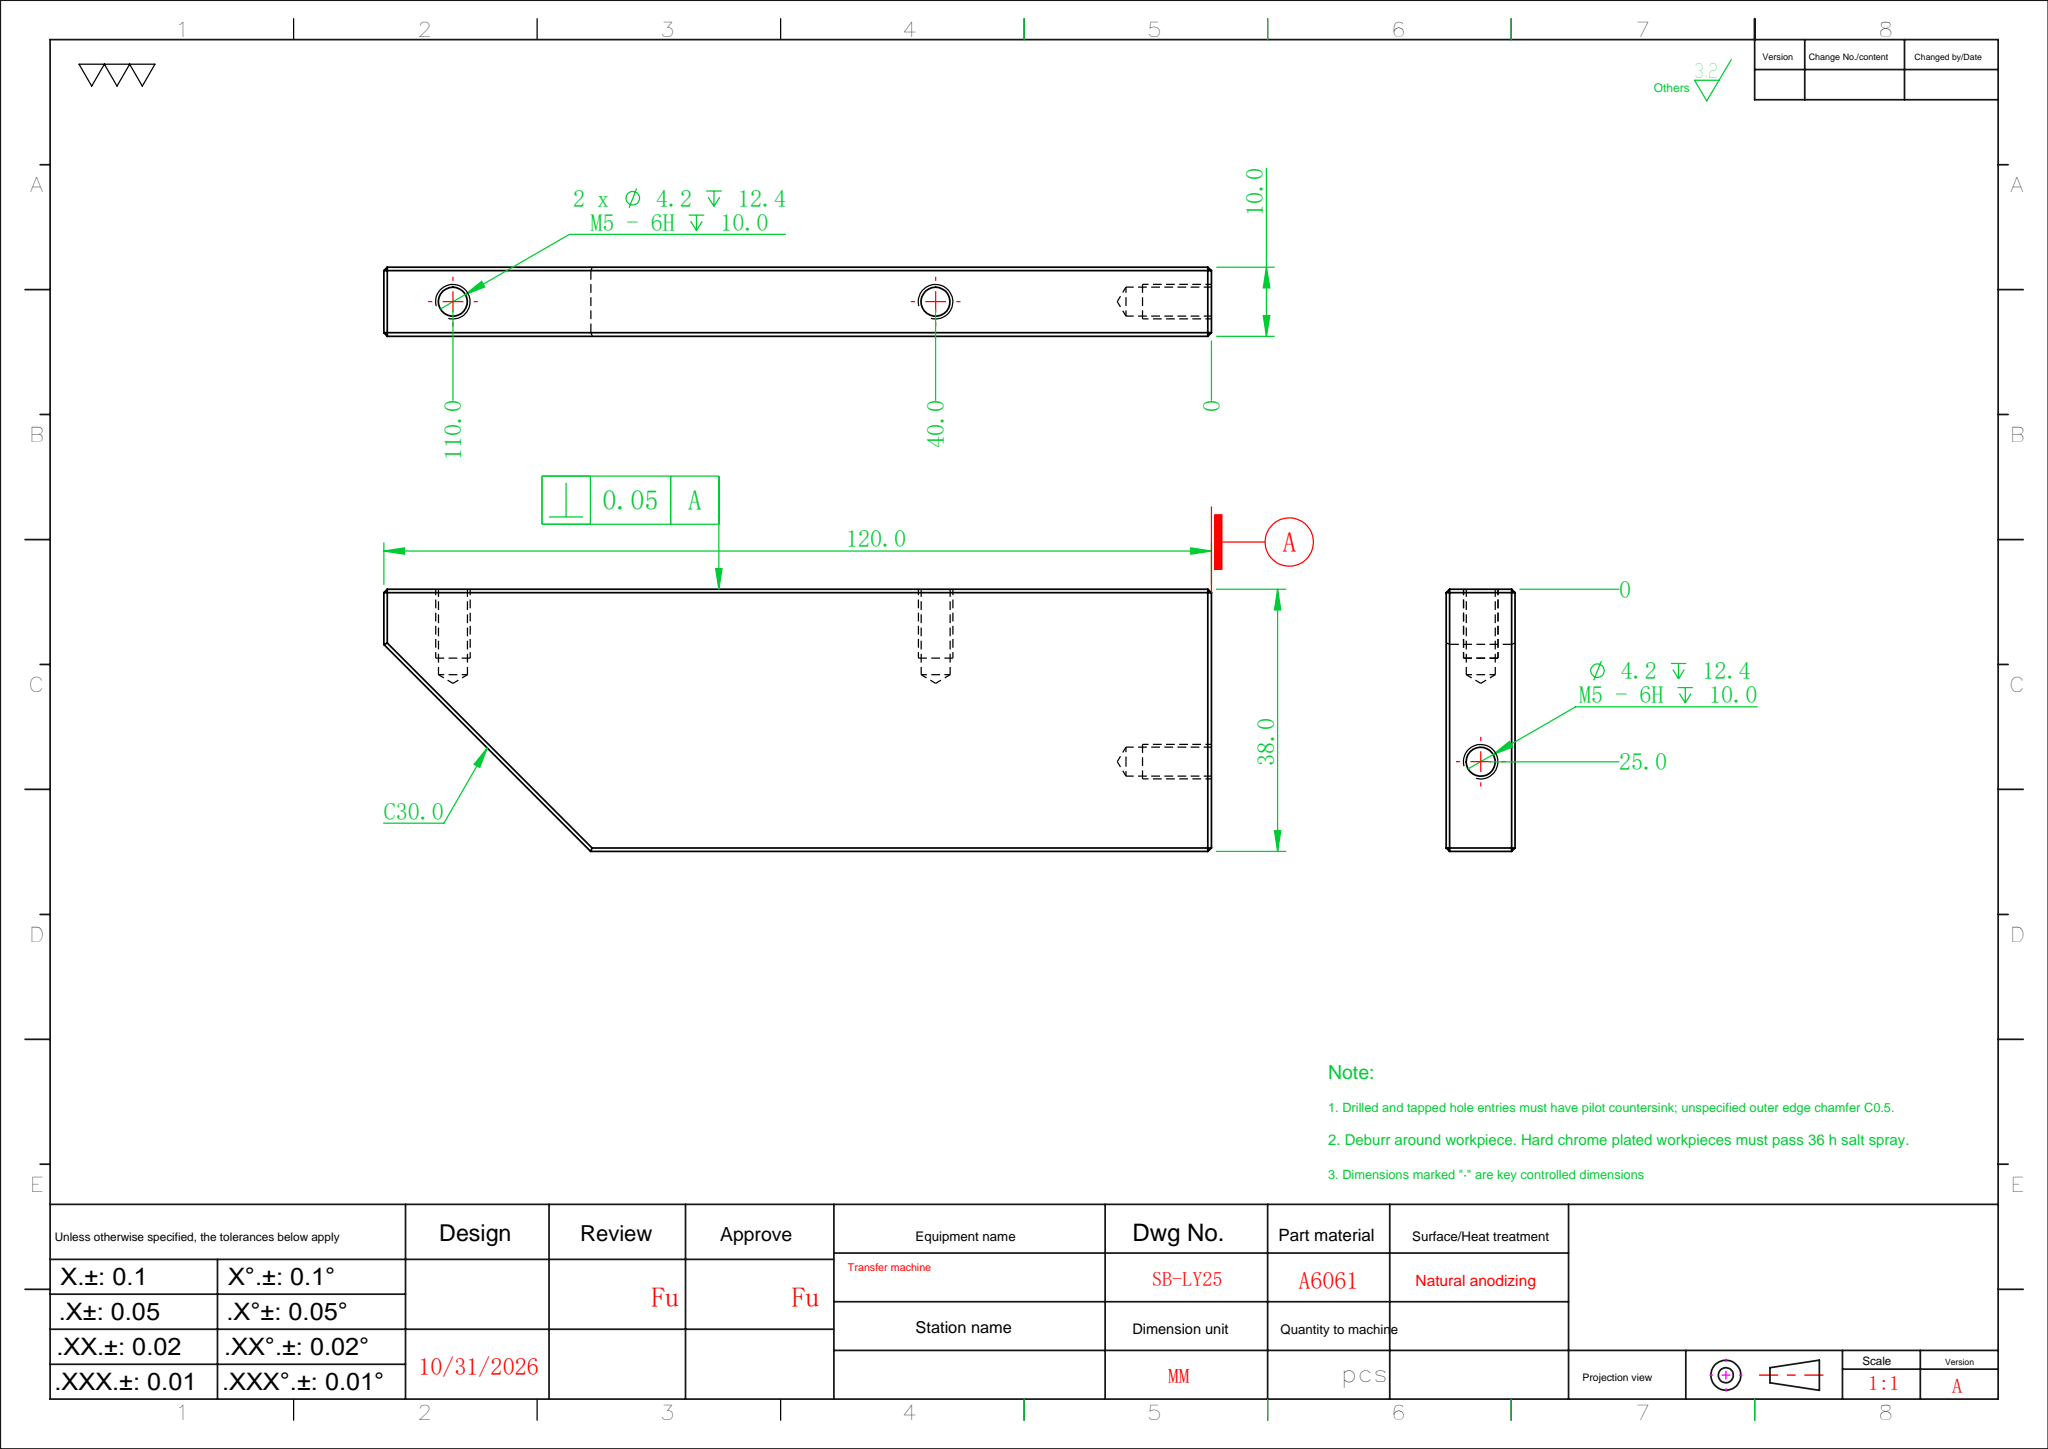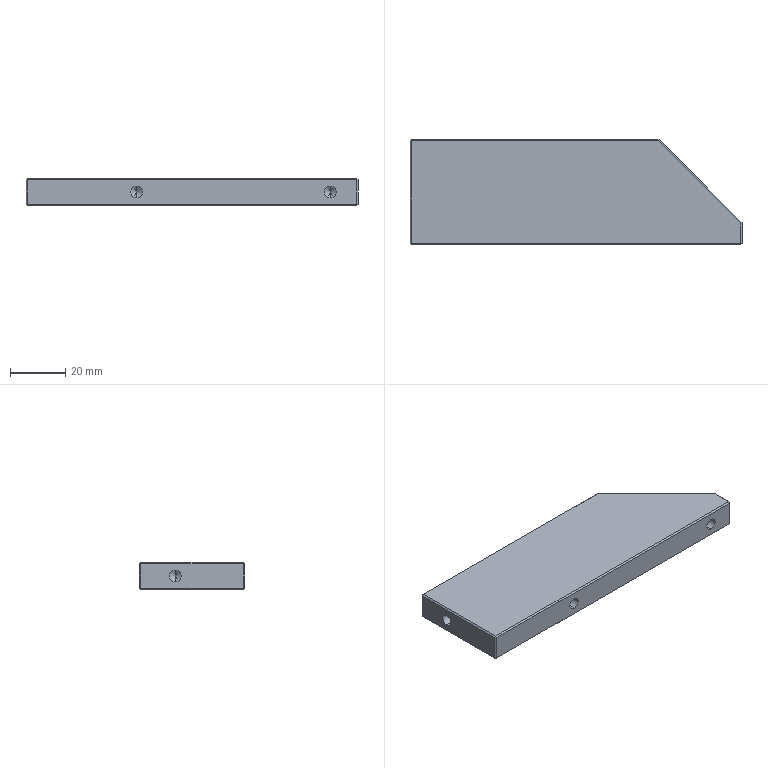Part | SolidWorks | features Chamfer 2, HoleWzd 2, Extrusion 1 | 1 solid | 38 faces | box 120 x 38 x 10 mm | volume 40489 mm3 | plane 26 | cylinder 6 | cone 6 | commonest cylinder face diameters 4.2 x6
STEP:
#1=CARTESIAN_POINT('',(50.,-6.6,7.1));
#2=VERTEX_POINT('',#1);
#3=CARTESIAN_POINT('',(50.,-6.6,2.9));
#4=VERTEX_POINT('',#3);
#5=CARTESIAN_POINT('',(50.,-6.6,5.));
#6=DIRECTION('',(0.,-1.,0.));
#7=DIRECTION('',(0.,0.,-1.));
#8=AXIS2_PLACEMENT_3D('',#5,#6,#7);
#9=CIRCLE('',#8,2.1);
#10=EDGE_CURVE('',#2,#4,#9,.T.);
#11=ORIENTED_EDGE('',*,*,#10,.F.);
#12=CARTESIAN_POINT('',(50.,-19.,7.1));
#13=VERTEX_POINT('',#12);
#14=CARTESIAN_POINT('',(50.,-19.,7.1));
#15=DIRECTION('',(0.,-1.,0.));
#16=VECTOR('',#15,1000.);
#17=LINE('',#14,#16);
#18=EDGE_CURVE('',#2,#13,#17,.T.);
#19=ORIENTED_EDGE('',*,*,#18,.T.);
#20=CARTESIAN_POINT('',(50.,-19.,2.9));
#21=VERTEX_POINT('',#20);
#22=CARTESIAN_POINT('',(50.,-19.,5.));
#23=DIRECTION('',(0.,-1.,0.));
#24=DIRECTION('',(0.,0.,-1.));
#25=AXIS2_PLACEMENT_3D('',#22,#23,#24);
#26=CIRCLE('',#25,2.1);
#27=EDGE_CURVE('',#13,#21,#26,.T.);
#28=ORIENTED_EDGE('',*,*,#27,.T.);
#29=CARTESIAN_POINT('',(50.,-19.,2.9));
#30=DIRECTION('',(0.,-1.,0.));
#31=VECTOR('',#30,1000.);
#32=LINE('',#29,#31);
#33=EDGE_CURVE('',#4,#21,#32,.T.);
#34=ORIENTED_EDGE('',*,*,#33,.F.);
#35=EDGE_LOOP('',(#11,#19,#28,#34));
#36=FACE_OUTER_BOUND('',#35,.T.);
#37=CARTESIAN_POINT('',(50.,-19.,5.));
#38=DIRECTION('',(0.,-1.,0.));
#39=DIRECTION('',(0.,0.,-1.));
#40=AXIS2_PLACEMENT_3D('',#37,#38,#39);
#41=CYLINDRICAL_SURFACE('',#40,2.1);
#42=ADVANCED_FACE('',(#36),#41,.F.);
#43=CARTESIAN_POINT('',(50.,-5.338,5.));
#44=VERTEX_POINT('',#43);
#45=CARTESIAN_POINT('',(50.,-6.6,2.9));
#46=DIRECTION('',(0.,-0.515,-0.8572));
#47=VECTOR('',#46,1000.);
#48=LINE('',#45,#47);
#49=EDGE_CURVE('',#44,#4,#48,.T.);
#50=ORIENTED_EDGE('',*,*,#49,.F.);
#51=CARTESIAN_POINT('',(50.,-6.6,7.1));
#52=DIRECTION('',(0.,-0.515,0.8572));
#53=VECTOR('',#52,1000.);
#54=LINE('',#51,#53);
#55=EDGE_CURVE('',#44,#2,#54,.T.);
#56=ORIENTED_EDGE('',*,*,#55,.T.);
#57=ORIENTED_EDGE('',*,*,#10,.T.);
#58=EDGE_LOOP('',(#50,#56,#57));
#59=FACE_OUTER_BOUND('',#58,.T.);
#60=CARTESIAN_POINT('',(50.,-6.6,5.));
#61=DIRECTION('',(0.,-1.,0.));
#62=DIRECTION('',(0.,0.,-1.));
#63=AXIS2_PLACEMENT_3D('',#60,#61,#62);
#64=CONICAL_SURFACE('',#63,2.1,1.03);
#65=ADVANCED_FACE('',(#59),#64,.F.);
#66=CARTESIAN_POINT('',(-20.,-6.6,7.1));
#67=VERTEX_POINT('',#66);
#68=CARTESIAN_POINT('',(-20.,-6.6,2.9));
#69=VERTEX_POINT('',#68);
#70=CARTESIAN_POINT('',(-20.,-6.6,5.));
#71=DIRECTION('',(0.,-1.,0.));
#72=DIRECTION('',(0.,0.,-1.));
#73=AXIS2_PLACEMENT_3D('',#70,#71,#72);
#74=CIRCLE('',#73,2.1);
#75=EDGE_CURVE('',#67,#69,#74,.T.);
#76=ORIENTED_EDGE('',*,*,#75,.F.);
#77=CARTESIAN_POINT('',(-20.,-19.,7.1));
#78=VERTEX_POINT('',#77);
#79=CARTESIAN_POINT('',(-20.,-19.,7.1));
#80=DIRECTION('',(0.,-1.,0.));
#81=VECTOR('',#80,1000.);
#82=LINE('',#79,#81);
#83=EDGE_CURVE('',#67,#78,#82,.T.);
#84=ORIENTED_EDGE('',*,*,#83,.T.);
#85=CARTESIAN_POINT('',(-20.,-19.,2.9));
#86=VERTEX_POINT('',#85);
#87=CARTESIAN_POINT('',(-20.,-19.,5.));
#88=DIRECTION('',(0.,-1.,0.));
#89=DIRECTION('',(0.,0.,-1.));
#90=AXIS2_PLACEMENT_3D('',#87,#88,#89);
#91=CIRCLE('',#90,2.1);
#92=EDGE_CURVE('',#78,#86,#91,.T.);
#93=ORIENTED_EDGE('',*,*,#92,.T.);
#94=CARTESIAN_POINT('',(-20.,-19.,2.9));
#95=DIRECTION('',(0.,-1.,0.));
#96=VECTOR('',#95,1000.);
#97=LINE('',#94,#96);
#98=EDGE_CURVE('',#69,#86,#97,.T.);
#99=ORIENTED_EDGE('',*,*,#98,.F.);
#100=EDGE_LOOP('',(#76,#84,#93,#99));
#101=FACE_OUTER_BOUND('',#100,.T.);
#102=CARTESIAN_POINT('',(-20.,-19.,5.));
#103=DIRECTION('',(0.,-1.,0.));
#104=DIRECTION('',(0.,0.,-1.));
#105=AXIS2_PLACEMENT_3D('',#102,#103,#104);
#106=CYLINDRICAL_SURFACE('',#105,2.1);
#107=ADVANCED_FACE('',(#101),#106,.F.);
#108=CARTESIAN_POINT('',(-20.,-5.338,5.));
#109=VERTEX_POINT('',#108);
#110=CARTESIAN_POINT('',(-20.,-6.6,2.9));
#111=DIRECTION('',(0.,-0.515,-0.8572));
#112=VECTOR('',#111,1000.);
#113=LINE('',#110,#112);
#114=EDGE_CURVE('',#109,#69,#113,.T.);
#115=ORIENTED_EDGE('',*,*,#114,.F.);
#116=CARTESIAN_POINT('',(-20.,-6.6,7.1));
#117=DIRECTION('',(0.,-0.515,0.8572));
#118=VECTOR('',#117,1000.);
#119=LINE('',#116,#118);
#120=EDGE_CURVE('',#109,#67,#119,.T.);
#121=ORIENTED_EDGE('',*,*,#120,.T.);
#122=ORIENTED_EDGE('',*,*,#75,.T.);
#123=EDGE_LOOP('',(#115,#121,#122));
#124=FACE_OUTER_BOUND('',#123,.T.);
#125=CARTESIAN_POINT('',(-20.,-6.6,5.));
#126=DIRECTION('',(0.,-1.,0.));
#127=DIRECTION('',(0.,0.,-1.));
#128=AXIS2_PLACEMENT_3D('',#125,#126,#127);
#129=CONICAL_SURFACE('',#128,2.1,1.03);
#130=ADVANCED_FACE('',(#124),#129,.F.);
#131=CARTESIAN_POINT('',(-47.6,6.,2.9));
#132=VERTEX_POINT('',#131);
#133=CARTESIAN_POINT('',(-47.6,6.,7.1));
#134=VERTEX_POINT('',#133);
#135=CARTESIAN_POINT('',(-47.6,6.,5.));
#136=DIRECTION('',(-1.,0.,0.));
#137=DIRECTION('',(0.,0.,1.));
#138=AXIS2_PLACEMENT_3D('',#135,#136,#137);
#139=CIRCLE('',#138,2.1);
#140=EDGE_CURVE('',#132,#134,#139,.T.);
#141=ORIENTED_EDGE('',*,*,#140,.F.);
#142=CARTESIAN_POINT('',(-60.,6.,2.9));
#143=VERTEX_POINT('',#142);
#144=CARTESIAN_POINT('',(-60.,6.,2.9));
#145=DIRECTION('',(-1.,0.,0.));
#146=VECTOR('',#145,1000.);
#147=LINE('',#144,#146);
#148=EDGE_CURVE('',#132,#143,#147,.T.);
#149=ORIENTED_EDGE('',*,*,#148,.T.);
#150=CARTESIAN_POINT('',(-60.,6.,7.1));
#151=VERTEX_POINT('',#150);
#152=CARTESIAN_POINT('',(-60.,6.,5.));
#153=DIRECTION('',(-1.,0.,0.));
#154=DIRECTION('',(0.,0.,1.));
#155=AXIS2_PLACEMENT_3D('',#152,#153,#154);
#156=CIRCLE('',#155,2.1);
#157=EDGE_CURVE('',#143,#151,#156,.T.);
#158=ORIENTED_EDGE('',*,*,#157,.T.);
#159=CARTESIAN_POINT('',(-60.,6.,7.1));
#160=DIRECTION('',(-1.,0.,0.));
#161=VECTOR('',#160,1000.);
#162=LINE('',#159,#161);
#163=EDGE_CURVE('',#134,#151,#162,.T.);
#164=ORIENTED_EDGE('',*,*,#163,.F.);
#165=EDGE_LOOP('',(#141,#149,#158,#164));
#166=FACE_OUTER_BOUND('',#165,.T.);
#167=CARTESIAN_POINT('',(-60.,6.,5.));
#168=DIRECTION('',(-1.,0.,0.));
#169=DIRECTION('',(0.,0.,1.));
#170=AXIS2_PLACEMENT_3D('',#167,#168,#169);
#171=CYLINDRICAL_SURFACE('',#170,2.1);
#172=ADVANCED_FACE('',(#166),#171,.F.);
#173=CARTESIAN_POINT('',(-46.338,6.,5.));
#174=VERTEX_POINT('',#173);
#175=CARTESIAN_POINT('',(-47.6,6.,7.1));
#176=DIRECTION('',(-0.515,0.,0.8572));
#177=VECTOR('',#176,1000.);
#178=LINE('',#175,#177);
#179=EDGE_CURVE('',#174,#134,#178,.T.);
#180=ORIENTED_EDGE('',*,*,#179,.F.);
#181=CARTESIAN_POINT('',(-47.6,6.,2.9));
#182=DIRECTION('',(-0.515,0.,-0.8572));
#183=VECTOR('',#182,1000.);
#184=LINE('',#181,#183);
#185=EDGE_CURVE('',#174,#132,#184,.T.);
#186=ORIENTED_EDGE('',*,*,#185,.T.);
#187=ORIENTED_EDGE('',*,*,#140,.T.);
#188=EDGE_LOOP('',(#180,#186,#187));
#189=FACE_OUTER_BOUND('',#188,.T.);
#190=CARTESIAN_POINT('',(-47.6,6.,5.));
#191=DIRECTION('',(-1.,0.,0.));
#192=DIRECTION('',(0.,0.,1.));
#193=AXIS2_PLACEMENT_3D('',#190,#191,#192);
#194=CONICAL_SURFACE('',#193,2.1,1.03);
#195=ADVANCED_FACE('',(#189),#194,.F.);
#196=CARTESIAN_POINT('',(60.,-11.,0.5));
#197=VERTEX_POINT('',#196);
#198=CARTESIAN_POINT('',(60.,-11.,9.5));
#199=VERTEX_POINT('',#198);
#200=CARTESIAN_POINT('',(60.,-11.,10.));
#201=DIRECTION('',(0.,0.,1.));
#202=VECTOR('',#201,1000.);
#203=LINE('',#200,#202);
#204=EDGE_CURVE('',#197,#199,#203,.T.);
#205=ORIENTED_EDGE('',*,*,#204,.T.);
#206=CARTESIAN_POINT('',(60.,-18.5,9.5));
#207=VERTEX_POINT('',#206);
#208=CARTESIAN_POINT('',(60.,-19.,9.5));
#209=DIRECTION('',(0.,-1.,0.));
#210=VECTOR('',#209,1000.);
#211=LINE('',#208,#210);
#212=EDGE_CURVE('',#199,#207,#211,.T.);
#213=ORIENTED_EDGE('',*,*,#212,.T.);
#214=CARTESIAN_POINT('',(60.,-18.5,0.5));
#215=VERTEX_POINT('',#214);
#216=CARTESIAN_POINT('',(60.,-18.5,10.));
#217=DIRECTION('',(0.,0.,-1.));
#218=VECTOR('',#217,1000.);
#219=LINE('',#216,#218);
#220=EDGE_CURVE('',#207,#215,#219,.T.);
#221=ORIENTED_EDGE('',*,*,#220,.T.);
#222=CARTESIAN_POINT('',(60.,-11.,0.5));
#223=DIRECTION('',(0.,1.,0.));
#224=VECTOR('',#223,1000.);
#225=LINE('',#222,#224);
#226=EDGE_CURVE('',#215,#197,#225,.T.);
#227=ORIENTED_EDGE('',*,*,#226,.T.);
#228=EDGE_LOOP('',(#205,#213,#221,#227));
#229=FACE_OUTER_BOUND('',#228,.T.);
#230=CARTESIAN_POINT('',(60.,-19.,10.));
#231=DIRECTION('',(-1.,0.,0.));
#232=DIRECTION('',(0.,0.,1.));
#233=AXIS2_PLACEMENT_3D('',#230,#231,#232);
#234=PLANE('',#233);
#235=ADVANCED_FACE('',(#229),#234,.F.);
#236=CARTESIAN_POINT('',(-59.5,19.,0.5));
#237=VERTEX_POINT('',#236);
#238=CARTESIAN_POINT('',(-59.5,19.,9.5));
#239=VERTEX_POINT('',#238);
#240=CARTESIAN_POINT('',(-59.5,19.,10.));
#241=DIRECTION('',(0.,0.,1.));
#242=VECTOR('',#241,1000.);
#243=LINE('',#240,#242);
#244=EDGE_CURVE('',#237,#239,#243,.T.);
#245=ORIENTED_EDGE('',*,*,#244,.T.);
#246=CARTESIAN_POINT('',(30.,19.,9.5));
#247=VERTEX_POINT('',#246);
#248=CARTESIAN_POINT('',(-60.,19.,9.5));
#249=DIRECTION('',(1.,0.,0.));
#250=VECTOR('',#249,1000.);
#251=LINE('',#248,#250);
#252=EDGE_CURVE('',#239,#247,#251,.T.);
#253=ORIENTED_EDGE('',*,*,#252,.T.);
#254=CARTESIAN_POINT('',(30.,19.,0.5));
#255=VERTEX_POINT('',#254);
#256=CARTESIAN_POINT('',(30.,19.,10.));
#257=DIRECTION('',(0.,0.,-1.));
#258=VECTOR('',#257,1000.);
#259=LINE('',#256,#258);
#260=EDGE_CURVE('',#247,#255,#259,.T.);
#261=ORIENTED_EDGE('',*,*,#260,.T.);
#262=CARTESIAN_POINT('',(-60.,19.,0.5));
#263=DIRECTION('',(-1.,0.,0.));
#264=VECTOR('',#263,1000.);
#265=LINE('',#262,#264);
#266=EDGE_CURVE('',#255,#237,#265,.T.);
#267=ORIENTED_EDGE('',*,*,#266,.T.);
#268=EDGE_LOOP('',(#245,#253,#261,#267));
#269=FACE_OUTER_BOUND('',#268,.T.);
#270=CARTESIAN_POINT('',(-60.,19.,10.));
#271=DIRECTION('',(0.,-1.,0.));
#272=DIRECTION('',(0.,0.,-1.));
#273=AXIS2_PLACEMENT_3D('',#270,#271,#272);
#274=PLANE('',#273);
#275=ADVANCED_FACE('',(#269),#274,.F.);
#276=CARTESIAN_POINT('',(-60.,18.5,0.5));
#277=VERTEX_POINT('',#276);
#278=CARTESIAN_POINT('',(-60.,-18.5,0.5));
#279=VERTEX_POINT('',#278);
#280=CARTESIAN_POINT('',(-60.,-19.,0.5));
#281=DIRECTION('',(0.,-1.,0.));
#282=VECTOR('',#281,1000.);
#283=LINE('',#280,#282);
#284=EDGE_CURVE('',#277,#279,#283,.T.);
#285=ORIENTED_EDGE('',*,*,#284,.T.);
#286=CARTESIAN_POINT('',(-60.,-18.5,9.5));
#287=VERTEX_POINT('',#286);
#288=CARTESIAN_POINT('',(-60.,-18.5,10.));
#289=DIRECTION('',(0.,0.,1.));
#290=VECTOR('',#289,1000.);
#291=LINE('',#288,#290);
#292=EDGE_CURVE('',#279,#287,#291,.T.);
#293=ORIENTED_EDGE('',*,*,#292,.T.);
#294=CARTESIAN_POINT('',(-60.,18.5,9.5));
#295=VERTEX_POINT('',#294);
#296=CARTESIAN_POINT('',(-60.,-19.,9.5));
#297=DIRECTION('',(0.,1.,0.));
#298=VECTOR('',#297,1000.);
#299=LINE('',#296,#298);
#300=EDGE_CURVE('',#287,#295,#299,.T.);
#301=ORIENTED_EDGE('',*,*,#300,.T.);
#302=CARTESIAN_POINT('',(-60.,18.5,10.));
#303=DIRECTION('',(0.,0.,-1.));
#304=VECTOR('',#303,1000.);
#305=LINE('',#302,#304);
#306=EDGE_CURVE('',#295,#277,#305,.T.);
#307=ORIENTED_EDGE('',*,*,#306,.T.);
#308=EDGE_LOOP('',(#285,#293,#301,#307));
#309=FACE_OUTER_BOUND('',#308,.T.);
#310=CARTESIAN_POINT('',(-60.,6.,5.));
#311=DIRECTION('',(-1.,0.,0.));
#312=DIRECTION('',(0.,0.,1.));
#313=AXIS2_PLACEMENT_3D('',#310,#311,#312);
#314=CIRCLE('',#313,2.1);
#315=EDGE_CURVE('',#151,#143,#314,.T.);
#316=ORIENTED_EDGE('',*,*,#315,.F.);
#317=ORIENTED_EDGE('',*,*,#157,.F.);
#318=EDGE_LOOP('',(#316,#317));
#319=FACE_BOUND('',#318,.T.);
#320=CARTESIAN_POINT('',(-60.,-19.,10.));
#321=DIRECTION('',(1.,0.,0.));
#322=DIRECTION('',(0.,0.,-1.));
#323=AXIS2_PLACEMENT_3D('',#320,#321,#322);
#324=PLANE('',#323);
#325=ADVANCED_FACE('',(#309,#319),#324,.F.);
#326=CARTESIAN_POINT('',(59.5,-19.,0.5));
#327=VERTEX_POINT('',#326);
#328=CARTESIAN_POINT('',(59.5,-19.,9.5));
#329=VERTEX_POINT('',#328);
#330=CARTESIAN_POINT('',(59.5,-19.,10.));
#331=DIRECTION('',(0.,0.,1.));
#332=VECTOR('',#331,1000.);
#333=LINE('',#330,#332);
#334=EDGE_CURVE('',#327,#329,#333,.T.);
#335=ORIENTED_EDGE('',*,*,#334,.T.);
#336=CARTESIAN_POINT('',(-59.5,-19.,9.5));
#337=VERTEX_POINT('',#336);
#338=CARTESIAN_POINT('',(-60.,-19.,9.5));
#339=DIRECTION('',(-1.,0.,0.));
#340=VECTOR('',#339,1000.);
#341=LINE('',#338,#340);
#342=EDGE_CURVE('',#329,#337,#341,.T.);
#343=ORIENTED_EDGE('',*,*,#342,.T.);
#344=CARTESIAN_POINT('',(-59.5,-19.,0.5));
#345=VERTEX_POINT('',#344);
#346=CARTESIAN_POINT('',(-59.5,-19.,10.));
#347=DIRECTION('',(0.,0.,-1.));
#348=VECTOR('',#347,1000.);
#349=LINE('',#346,#348);
#350=EDGE_CURVE('',#337,#345,#349,.T.);
#351=ORIENTED_EDGE('',*,*,#350,.T.);
#352=CARTESIAN_POINT('',(60.,-19.,0.5));
#353=DIRECTION('',(1.,0.,0.));
#354=VECTOR('',#353,1000.);
#355=LINE('',#352,#354);
#356=EDGE_CURVE('',#345,#327,#355,.T.);
#357=ORIENTED_EDGE('',*,*,#356,.T.);
#358=EDGE_LOOP('',(#335,#343,#351,#357));
#359=FACE_OUTER_BOUND('',#358,.T.);
#360=CARTESIAN_POINT('',(50.,-19.,5.));
#361=DIRECTION('',(0.,-1.,0.));
#362=DIRECTION('',(0.,0.,-1.));
#363=AXIS2_PLACEMENT_3D('',#360,#361,#362);
#364=CIRCLE('',#363,2.1);
#365=EDGE_CURVE('',#21,#13,#364,.T.);
#366=ORIENTED_EDGE('',*,*,#365,.F.);
#367=ORIENTED_EDGE('',*,*,#27,.F.);
#368=EDGE_LOOP('',(#366,#367));
#369=FACE_BOUND('',#368,.T.);
#370=CARTESIAN_POINT('',(-20.,-19.,5.));
#371=DIRECTION('',(0.,-1.,0.));
#372=DIRECTION('',(0.,0.,-1.));
#373=AXIS2_PLACEMENT_3D('',#370,#371,#372);
#374=CIRCLE('',#373,2.1);
#375=EDGE_CURVE('',#86,#78,#374,.T.);
#376=ORIENTED_EDGE('',*,*,#375,.F.);
#377=ORIENTED_EDGE('',*,*,#92,.F.);
#378=EDGE_LOOP('',(#376,#377));
#379=FACE_BOUND('',#378,.T.);
#380=CARTESIAN_POINT('',(-60.,-19.,10.));
#381=DIRECTION('',(0.,1.,0.));
#382=DIRECTION('',(0.,0.,1.));
#383=AXIS2_PLACEMENT_3D('',#380,#381,#382);
#384=PLANE('',#383);
#385=ADVANCED_FACE('',(#359,#369,#379),#384,.F.);
#386=CARTESIAN_POINT('',(-59.5,18.5,10.));
#387=VERTEX_POINT('',#386);
#388=CARTESIAN_POINT('',(-59.5,-18.5,10.));
#389=VERTEX_POINT('',#388);
#390=CARTESIAN_POINT('',(-59.5,0.,10.));
#391=DIRECTION('',(0.,-1.,0.));
#392=VECTOR('',#391,1000.);
#393=LINE('',#390,#392);
#394=EDGE_CURVE('',#387,#389,#393,.T.);
#395=ORIENTED_EDGE('',*,*,#394,.T.);
#396=CARTESIAN_POINT('',(59.5,-18.5,10.));
#397=VERTEX_POINT('',#396);
#398=CARTESIAN_POINT('',(0.,-18.5,10.));
#399=DIRECTION('',(1.,0.,0.));
#400=VECTOR('',#399,1000.);
#401=LINE('',#398,#400);
#402=EDGE_CURVE('',#389,#397,#401,.T.);
#403=ORIENTED_EDGE('',*,*,#402,.T.);
#404=CARTESIAN_POINT('',(59.5,-11.207,10.));
#405=VERTEX_POINT('',#404);
#406=CARTESIAN_POINT('',(59.5,0.,10.));
#407=DIRECTION('',(0.,1.,0.));
#408=VECTOR('',#407,1000.);
#409=LINE('',#406,#408);
#410=EDGE_CURVE('',#397,#405,#409,.T.);
#411=ORIENTED_EDGE('',*,*,#410,.T.);
#412=CARTESIAN_POINT('',(29.793,18.5,10.));
#413=VERTEX_POINT('',#412);
#414=CARTESIAN_POINT('',(29.646,18.646,10.));
#415=DIRECTION('',(-0.7071,0.7071,0.));
#416=VECTOR('',#415,1000.);
#417=LINE('',#414,#416);
#418=EDGE_CURVE('',#405,#413,#417,.T.);
#419=ORIENTED_EDGE('',*,*,#418,.T.);
#420=CARTESIAN_POINT('',(0.,18.5,10.));
#421=DIRECTION('',(-1.,0.,0.));
#422=VECTOR('',#421,1000.);
#423=LINE('',#420,#422);
#424=EDGE_CURVE('',#413,#387,#423,.T.);
#425=ORIENTED_EDGE('',*,*,#424,.T.);
#426=EDGE_LOOP('',(#395,#403,#411,#419,#425));
#427=FACE_OUTER_BOUND('',#426,.T.);
#428=CARTESIAN_POINT('',(0.,0.,10.));
#429=DIRECTION('',(0.,0.,-1.));
#430=DIRECTION('',(-1.,0.,0.));
#431=AXIS2_PLACEMENT_3D('',#428,#429,#430);
#432=PLANE('',#431);
#433=ADVANCED_FACE('',(#427),#432,.F.);
#434=CARTESIAN_POINT('',(59.5,-18.5,0.));
#435=VERTEX_POINT('',#434);
#436=CARTESIAN_POINT('',(-59.5,-18.5,0.));
#437=VERTEX_POINT('',#436);
#438=CARTESIAN_POINT('',(-60.,-18.5,0.));
#439=DIRECTION('',(-1.,0.,0.));
#440=VECTOR('',#439,1000.);
#441=LINE('',#438,#440);
#442=EDGE_CURVE('',#435,#437,#441,.T.);
#443=ORIENTED_EDGE('',*,*,#442,.T.);
#444=CARTESIAN_POINT('',(-59.5,18.5,0.));
#445=VERTEX_POINT('',#444);
#446=CARTESIAN_POINT('',(-59.5,19.,0.));
#447=DIRECTION('',(0.,1.,0.));
#448=VECTOR('',#447,1000.);
#449=LINE('',#446,#448);
#450=EDGE_CURVE('',#437,#445,#449,.T.);
#451=ORIENTED_EDGE('',*,*,#450,.T.);
#452=CARTESIAN_POINT('',(29.793,18.5,0.));
#453=VERTEX_POINT('',#452);
#454=CARTESIAN_POINT('',(30.,18.5,0.));
#455=DIRECTION('',(1.,0.,0.));
#456=VECTOR('',#455,1000.);
#457=LINE('',#454,#456);
#458=EDGE_CURVE('',#445,#453,#457,.T.);
#459=ORIENTED_EDGE('',*,*,#458,.T.);
#460=CARTESIAN_POINT('',(59.5,-11.207,0.));
#461=VERTEX_POINT('',#460);
#462=CARTESIAN_POINT('',(24.146,24.146,0.));
#463=DIRECTION('',(0.7071,-0.7071,0.));
#464=VECTOR('',#463,1000.);
#465=LINE('',#462,#464);
#466=EDGE_CURVE('',#453,#461,#465,.T.);
#467=ORIENTED_EDGE('',*,*,#466,.T.);
#468=CARTESIAN_POINT('',(59.5,-19.,0.));
#469=DIRECTION('',(0.,-1.,0.));
#470=VECTOR('',#469,1000.);
#471=LINE('',#468,#470);
#472=EDGE_CURVE('',#461,#435,#471,.T.);
#473=ORIENTED_EDGE('',*,*,#472,.T.);
#474=EDGE_LOOP('',(#443,#451,#459,#467,#473));
#475=FACE_OUTER_BOUND('',#474,.T.);
#476=CARTESIAN_POINT('',(0.,0.,0.));
#477=DIRECTION('',(0.,0.,-1.));
#478=DIRECTION('',(-1.,0.,0.));
#479=AXIS2_PLACEMENT_3D('',#476,#477,#478);
#480=PLANE('',#479);
#481=ADVANCED_FACE('',(#475),#480,.T.);
#482=ORIENTED_EDGE('',*,*,#260,.F.);
#483=CARTESIAN_POINT('',(60.,-11.,9.5));
#484=DIRECTION('',(0.7071,-0.7071,0.));
#485=VECTOR('',#484,1000.);
#486=LINE('',#483,#485);
#487=EDGE_CURVE('',#247,#199,#486,.T.);
#488=ORIENTED_EDGE('',*,*,#487,.T.);
#489=ORIENTED_EDGE('',*,*,#204,.F.);
#490=CARTESIAN_POINT('',(30.,19.,0.5));
#491=DIRECTION('',(-0.7071,0.7071,0.));
#492=VECTOR('',#491,1000.);
#493=LINE('',#490,#492);
#494=EDGE_CURVE('',#197,#255,#493,.T.);
#495=ORIENTED_EDGE('',*,*,#494,.T.);
#496=EDGE_LOOP('',(#482,#488,#489,#495));
#497=FACE_OUTER_BOUND('',#496,.T.);
#498=CARTESIAN_POINT('',(30.,19.,10.));
#499=DIRECTION('',(-0.7071,-0.7071,0.));
#500=DIRECTION('',(0.,0.,-1.));
#501=AXIS2_PLACEMENT_3D('',#498,#499,#500);
#502=PLANE('',#501);
#503=ADVANCED_FACE('',(#497),#502,.F.);
#504=ORIENTED_EDGE('',*,*,#185,.F.);
#505=ORIENTED_EDGE('',*,*,#179,.T.);
#506=CARTESIAN_POINT('',(-47.6,6.,5.));
#507=DIRECTION('',(-1.,0.,0.));
#508=DIRECTION('',(0.,0.,1.));
#509=AXIS2_PLACEMENT_3D('',#506,#507,#508);
#510=CIRCLE('',#509,2.1);
#511=EDGE_CURVE('',#134,#132,#510,.T.);
#512=ORIENTED_EDGE('',*,*,#511,.T.);
#513=EDGE_LOOP('',(#504,#505,#512));
#514=FACE_OUTER_BOUND('',#513,.T.);
#515=CARTESIAN_POINT('',(-47.6,6.,5.));
#516=DIRECTION('',(-1.,0.,0.));
#517=DIRECTION('',(0.,0.,1.));
#518=AXIS2_PLACEMENT_3D('',#515,#516,#517);
#519=CONICAL_SURFACE('',#518,2.1,1.03);
#520=ADVANCED_FACE('',(#514),#519,.F.);
#521=ORIENTED_EDGE('',*,*,#148,.F.);
#522=ORIENTED_EDGE('',*,*,#511,.F.);
#523=ORIENTED_EDGE('',*,*,#163,.T.);
#524=ORIENTED_EDGE('',*,*,#315,.T.);
#525=EDGE_LOOP('',(#521,#522,#523,#524));
#526=FACE_OUTER_BOUND('',#525,.T.);
#527=CARTESIAN_POINT('',(-60.,6.,5.));
#528=DIRECTION('',(-1.,0.,0.));
#529=DIRECTION('',(0.,0.,1.));
#530=AXIS2_PLACEMENT_3D('',#527,#528,#529);
#531=CYLINDRICAL_SURFACE('',#530,2.1);
#532=ADVANCED_FACE('',(#526),#531,.F.);
#533=ORIENTED_EDGE('',*,*,#120,.F.);
#534=ORIENTED_EDGE('',*,*,#114,.T.);
#535=CARTESIAN_POINT('',(-20.,-6.6,5.));
#536=DIRECTION('',(0.,-1.,0.));
#537=DIRECTION('',(0.,0.,-1.));
#538=AXIS2_PLACEMENT_3D('',#535,#536,#537);
#539=CIRCLE('',#538,2.1);
#540=EDGE_CURVE('',#69,#67,#539,.T.);
#541=ORIENTED_EDGE('',*,*,#540,.T.);
#542=EDGE_LOOP('',(#533,#534,#541));
#543=FACE_OUTER_BOUND('',#542,.T.);
#544=CARTESIAN_POINT('',(-20.,-6.6,5.));
#545=DIRECTION('',(0.,-1.,0.));
#546=DIRECTION('',(0.,0.,-1.));
#547=AXIS2_PLACEMENT_3D('',#544,#545,#546);
#548=CONICAL_SURFACE('',#547,2.1,1.03);
#549=ADVANCED_FACE('',(#543),#548,.F.);
#550=ORIENTED_EDGE('',*,*,#83,.F.);
#551=ORIENTED_EDGE('',*,*,#540,.F.);
#552=ORIENTED_EDGE('',*,*,#98,.T.);
#553=ORIENTED_EDGE('',*,*,#375,.T.);
#554=EDGE_LOOP('',(#550,#551,#552,#553));
#555=FACE_OUTER_BOUND('',#554,.T.);
#556=CARTESIAN_POINT('',(-20.,-19.,5.));
#557=DIRECTION('',(0.,-1.,0.));
#558=DIRECTION('',(0.,0.,-1.));
#559=AXIS2_PLACEMENT_3D('',#556,#557,#558);
#560=CYLINDRICAL_SURFACE('',#559,2.1);
#561=ADVANCED_FACE('',(#555),#560,.F.);
#562=ORIENTED_EDGE('',*,*,#55,.F.);
#563=ORIENTED_EDGE('',*,*,#49,.T.);
#564=CARTESIAN_POINT('',(50.,-6.6,5.));
#565=DIRECTION('',(0.,-1.,0.));
#566=DIRECTION('',(0.,0.,-1.));
#567=AXIS2_PLACEMENT_3D('',#564,#565,#566);
#568=CIRCLE('',#567,2.1);
#569=EDGE_CURVE('',#4,#2,#568,.T.);
#570=ORIENTED_EDGE('',*,*,#569,.T.);
#571=EDGE_LOOP('',(#562,#563,#570));
#572=FACE_OUTER_BOUND('',#571,.T.);
#573=CARTESIAN_POINT('',(50.,-6.6,5.));
#574=DIRECTION('',(0.,-1.,0.));
#575=DIRECTION('',(0.,0.,-1.));
#576=AXIS2_PLACEMENT_3D('',#573,#574,#575);
#577=CONICAL_SURFACE('',#576,2.1,1.03);
#578=ADVANCED_FACE('',(#572),#577,.F.);
#579=ORIENTED_EDGE('',*,*,#18,.F.);
#580=ORIENTED_EDGE('',*,*,#569,.F.);
#581=ORIENTED_EDGE('',*,*,#33,.T.);
#582=ORIENTED_EDGE('',*,*,#365,.T.);
#583=EDGE_LOOP('',(#579,#580,#581,#582));
#584=FACE_OUTER_BOUND('',#583,.T.);
#585=CARTESIAN_POINT('',(50.,-19.,5.));
#586=DIRECTION('',(0.,-1.,0.));
#587=DIRECTION('',(0.,0.,-1.));
#588=AXIS2_PLACEMENT_3D('',#585,#586,#587);
#589=CYLINDRICAL_SURFACE('',#588,2.1);
#590=ADVANCED_FACE('',(#584),#589,.F.);
#591=CARTESIAN_POINT('',(49.963,-15.157,19.537));
#592=DIRECTION('',(-0.6786,-0.2811,0.6786));
#593=VECTOR('',#592,1000.);
#594=LINE('',#591,#593);
#595=EDGE_CURVE('',#199,#405,#594,.T.);
#596=ORIENTED_EDGE('',*,*,#595,.F.);
#597=ORIENTED_EDGE('',*,*,#487,.F.);
#598=CARTESIAN_POINT('',(27.439,12.817,15.683));
#599=DIRECTION('',(0.2811,0.6786,-0.6786));
#600=VECTOR('',#599,1000.);
#601=LINE('',#598,#600);
#602=EDGE_CURVE('',#413,#247,#601,.T.);
#603=ORIENTED_EDGE('',*,*,#602,.F.);
#604=ORIENTED_EDGE('',*,*,#418,.F.);
#605=EDGE_LOOP('',(#596,#597,#603,#604));
#606=FACE_OUTER_BOUND('',#605,.T.);
#607=CARTESIAN_POINT('',(24.146,24.146,10.));
#608=DIRECTION('',(-0.5,-0.5,-0.7071));
#609=DIRECTION('',(-0.7071,0.7071,0.));
#610=AXIS2_PLACEMENT_3D('',#607,#608,#609);
#611=PLANE('',#610);
#612=ADVANCED_FACE('',(#606),#611,.F.);
#613=CARTESIAN_POINT('',(22.889,1.833,-16.667));
#614=DIRECTION('',(-0.2811,-0.6786,-0.6786));
#615=VECTOR('',#614,1000.);
#616=LINE('',#613,#615);
#617=EDGE_CURVE('',#255,#453,#616,.T.);
#618=ORIENTED_EDGE('',*,*,#617,.F.);
#619=ORIENTED_EDGE('',*,*,#494,.F.);
#620=CARTESIAN_POINT('',(49.963,-15.157,-9.537));
#621=DIRECTION('',(0.6786,0.2811,0.6786));
#622=VECTOR('',#621,1000.);
#623=LINE('',#620,#622);
#624=EDGE_CURVE('',#461,#197,#623,.T.);
#625=ORIENTED_EDGE('',*,*,#624,.F.);
#626=ORIENTED_EDGE('',*,*,#466,.F.);
#627=EDGE_LOOP('',(#618,#619,#625,#626));
#628=FACE_OUTER_BOUND('',#627,.T.);
#629=CARTESIAN_POINT('',(24.146,24.146,0.));
#630=DIRECTION('',(0.5,0.5,-0.7071));
#631=DIRECTION('',(-0.7071,0.7071,0.));
#632=AXIS2_PLACEMENT_3D('',#629,#630,#631);
#633=PLANE('',#632);
#634=ADVANCED_FACE('',(#628),#633,.T.);
#635=ORIENTED_EDGE('',*,*,#602,.T.);
#636=ORIENTED_EDGE('',*,*,#252,.F.);
#637=CARTESIAN_POINT('',(-59.5,18.75,9.75));
#638=DIRECTION('',(0.,0.7071,-0.7071));
#639=VECTOR('',#638,1000.);
#640=LINE('',#637,#639);
#641=EDGE_CURVE('',#387,#239,#640,.T.);
#642=ORIENTED_EDGE('',*,*,#641,.F.);
#643=ORIENTED_EDGE('',*,*,#424,.F.);
#644=EDGE_LOOP('',(#635,#636,#642,#643));
#645=FACE_OUTER_BOUND('',#644,.T.);
#646=CARTESIAN_POINT('',(0.,18.5,10.));
#647=DIRECTION('',(0.,-0.7071,-0.7071));
#648=DIRECTION('',(-1.,0.,0.));
#649=AXIS2_PLACEMENT_3D('',#646,#647,#648);
#650=PLANE('',#649);
#651=ADVANCED_FACE('',(#645),#650,.F.);
#652=ORIENTED_EDGE('',*,*,#595,.T.);
#653=ORIENTED_EDGE('',*,*,#410,.F.);
#654=CARTESIAN_POINT('',(59.75,-18.5,9.75));
#655=DIRECTION('',(-0.7071,0.,0.7071));
#656=VECTOR('',#655,1000.);
#657=LINE('',#654,#656);
#658=EDGE_CURVE('',#207,#397,#657,.T.);
#659=ORIENTED_EDGE('',*,*,#658,.F.);
#660=ORIENTED_EDGE('',*,*,#212,.F.);
#661=EDGE_LOOP('',(#652,#653,#659,#660));
#662=FACE_OUTER_BOUND('',#661,.T.);
#663=CARTESIAN_POINT('',(59.5,0.,10.));
#664=DIRECTION('',(-0.7071,0.,-0.7071));
#665=DIRECTION('',(0.,1.,0.));
#666=AXIS2_PLACEMENT_3D('',#663,#664,#665);
#667=PLANE('',#666);
#668=ADVANCED_FACE('',(#662),#667,.F.);
#669=CARTESIAN_POINT('',(60.,-18.5,0.5));
#670=DIRECTION('',(-0.7071,-0.7071,0.));
#671=VECTOR('',#670,1000.);
#672=LINE('',#669,#671);
#673=EDGE_CURVE('',#215,#327,#672,.T.);
#674=ORIENTED_EDGE('',*,*,#673,.F.);
#675=ORIENTED_EDGE('',*,*,#220,.F.);
#676=CARTESIAN_POINT('',(59.5,-19.,9.5));
#677=DIRECTION('',(0.7071,0.7071,0.));
#678=VECTOR('',#677,1000.);
#679=LINE('',#676,#678);
#680=EDGE_CURVE('',#329,#207,#679,.T.);
#681=ORIENTED_EDGE('',*,*,#680,.F.);
#682=ORIENTED_EDGE('',*,*,#334,.F.);
#683=EDGE_LOOP('',(#674,#675,#681,#682));
#684=FACE_OUTER_BOUND('',#683,.T.);
#685=CARTESIAN_POINT('',(60.,-18.5,10.));
#686=DIRECTION('',(-0.7071,0.7071,0.));
#687=DIRECTION('',(0.,0.,-1.));
#688=AXIS2_PLACEMENT_3D('',#685,#686,#687);
#689=PLANE('',#688);
#690=ADVANCED_FACE('',(#684),#689,.F.);
#691=ORIENTED_EDGE('',*,*,#624,.T.);
#692=ORIENTED_EDGE('',*,*,#226,.F.);
#693=CARTESIAN_POINT('',(60.,-18.5,0.5));
#694=DIRECTION('',(0.7071,0.,0.7071));
#695=VECTOR('',#694,1000.);
#696=LINE('',#693,#695);
#697=EDGE_CURVE('',#435,#215,#696,.T.);
#698=ORIENTED_EDGE('',*,*,#697,.F.);
#699=ORIENTED_EDGE('',*,*,#472,.F.);
#700=EDGE_LOOP('',(#691,#692,#698,#699));
#701=FACE_OUTER_BOUND('',#700,.T.);
#702=CARTESIAN_POINT('',(60.,-19.,0.5));
#703=DIRECTION('',(0.7071,0.,-0.7071));
#704=DIRECTION('',(0.,-1.,0.));
#705=AXIS2_PLACEMENT_3D('',#702,#703,#704);
#706=PLANE('',#705);
#707=ADVANCED_FACE('',(#701),#706,.T.);
#708=ORIENTED_EDGE('',*,*,#617,.T.);
#709=ORIENTED_EDGE('',*,*,#458,.F.);
#710=CARTESIAN_POINT('',(-59.5,18.5,0.));
#711=DIRECTION('',(0.,-0.7071,-0.7071));
#712=VECTOR('',#711,1000.);
#713=LINE('',#710,#712);
#714=EDGE_CURVE('',#237,#445,#713,.T.);
#715=ORIENTED_EDGE('',*,*,#714,.F.);
#716=ORIENTED_EDGE('',*,*,#266,.F.);
#717=EDGE_LOOP('',(#708,#709,#715,#716));
#718=FACE_OUTER_BOUND('',#717,.T.);
#719=CARTESIAN_POINT('',(-60.,19.,0.5));
#720=DIRECTION('',(0.,0.7071,-0.7071));
#721=DIRECTION('',(1.,0.,0.));
#722=AXIS2_PLACEMENT_3D('',#719,#720,#721);
#723=PLANE('',#722);
#724=ADVANCED_FACE('',(#718),#723,.T.);
#725=CARTESIAN_POINT('',(-60.,18.5,9.5));
#726=DIRECTION('',(-0.7071,-0.7071,0.));
#727=VECTOR('',#726,1000.);
#728=LINE('',#725,#727);
#729=EDGE_CURVE('',#239,#295,#728,.T.);
#730=ORIENTED_EDGE('',*,*,#729,.F.);
#731=ORIENTED_EDGE('',*,*,#244,.F.);
#732=CARTESIAN_POINT('',(-59.75,18.75,0.5));
#733=DIRECTION('',(0.7071,0.7071,0.));
#734=VECTOR('',#733,1000.);
#735=LINE('',#732,#734);
#736=EDGE_CURVE('',#277,#237,#735,.T.);
#737=ORIENTED_EDGE('',*,*,#736,.F.);
#738=ORIENTED_EDGE('',*,*,#306,.F.);
#739=EDGE_LOOP('',(#730,#731,#737,#738));
#740=FACE_OUTER_BOUND('',#739,.T.);
#741=CARTESIAN_POINT('',(-60.,18.5,10.));
#742=DIRECTION('',(0.7071,-0.7071,0.));
#743=DIRECTION('',(0.,0.,-1.));
#744=AXIS2_PLACEMENT_3D('',#741,#742,#743);
#745=PLANE('',#744);
#746=ADVANCED_FACE('',(#740),#745,.F.);
#747=ORIENTED_EDGE('',*,*,#641,.T.);
#748=ORIENTED_EDGE('',*,*,#729,.T.);
#749=CARTESIAN_POINT('',(-60.,18.5,9.5));
#750=DIRECTION('',(-0.7071,0.,-0.7071));
#751=VECTOR('',#750,1000.);
#752=LINE('',#749,#751);
#753=EDGE_CURVE('',#387,#295,#752,.T.);
#754=ORIENTED_EDGE('',*,*,#753,.F.);
#755=EDGE_LOOP('',(#747,#748,#754));
#756=FACE_OUTER_BOUND('',#755,.T.);
#757=CARTESIAN_POINT('',(-60.,18.5,9.5));
#758=DIRECTION('',(-0.5774,0.5774,0.5774));
#759=DIRECTION('',(0.7071,0.,0.7071));
#760=AXIS2_PLACEMENT_3D('',#757,#758,#759);
#761=PLANE('',#760);
#762=ADVANCED_FACE('',(#756),#761,.T.);
#763=ORIENTED_EDGE('',*,*,#680,.T.);
#764=ORIENTED_EDGE('',*,*,#658,.T.);
#765=CARTESIAN_POINT('',(59.5,-19.,9.5));
#766=DIRECTION('',(0.,0.7071,0.7071));
#767=VECTOR('',#766,1000.);
#768=LINE('',#765,#767);
#769=EDGE_CURVE('',#329,#397,#768,.T.);
#770=ORIENTED_EDGE('',*,*,#769,.F.);
#771=EDGE_LOOP('',(#763,#764,#770));
#772=FACE_OUTER_BOUND('',#771,.T.);
#773=CARTESIAN_POINT('',(59.5,-19.,9.5));
#774=DIRECTION('',(0.5774,-0.5774,0.5774));
#775=DIRECTION('',(0.7071,0.,-0.7071));
#776=AXIS2_PLACEMENT_3D('',#773,#774,#775);
#777=PLANE('',#776);
#778=ADVANCED_FACE('',(#772),#777,.T.);
#779=ORIENTED_EDGE('',*,*,#697,.T.);
#780=ORIENTED_EDGE('',*,*,#673,.T.);
#781=CARTESIAN_POINT('',(59.5,-18.75,0.25));
#782=DIRECTION('',(0.,-0.7071,0.7071));
#783=VECTOR('',#782,1000.);
#784=LINE('',#781,#783);
#785=EDGE_CURVE('',#435,#327,#784,.T.);
#786=ORIENTED_EDGE('',*,*,#785,.F.);
#787=EDGE_LOOP('',(#779,#780,#786));
#788=FACE_OUTER_BOUND('',#787,.T.);
#789=CARTESIAN_POINT('',(60.,-18.5,0.5));
#790=DIRECTION('',(0.5774,-0.5774,-0.5774));
#791=DIRECTION('',(-0.7071,0.,-0.7071));
#792=AXIS2_PLACEMENT_3D('',#789,#790,#791);
#793=PLANE('',#792);
#794=ADVANCED_FACE('',(#788),#793,.T.);
#795=ORIENTED_EDGE('',*,*,#736,.T.);
#796=ORIENTED_EDGE('',*,*,#714,.T.);
#797=CARTESIAN_POINT('',(-59.5,18.5,0.));
#798=DIRECTION('',(0.7071,0.,-0.7071));
#799=VECTOR('',#798,1000.);
#800=LINE('',#797,#799);
#801=EDGE_CURVE('',#277,#445,#800,.T.);
#802=ORIENTED_EDGE('',*,*,#801,.F.);
#803=EDGE_LOOP('',(#795,#796,#802));
#804=FACE_OUTER_BOUND('',#803,.T.);
#805=CARTESIAN_POINT('',(-59.5,18.5,0.));
#806=DIRECTION('',(-0.5774,0.5774,-0.5774));
#807=DIRECTION('',(-0.7071,0.,0.7071));
#808=AXIS2_PLACEMENT_3D('',#805,#806,#807);
#809=PLANE('',#808);
#810=ADVANCED_FACE('',(#804),#809,.T.);
#811=ORIENTED_EDGE('',*,*,#753,.T.);
#812=ORIENTED_EDGE('',*,*,#300,.F.);
#813=CARTESIAN_POINT('',(-60.,-18.5,9.5));
#814=DIRECTION('',(-0.7071,0.,-0.7071));
#815=VECTOR('',#814,1000.);
#816=LINE('',#813,#815);
#817=EDGE_CURVE('',#389,#287,#816,.T.);
#818=ORIENTED_EDGE('',*,*,#817,.F.);
#819=ORIENTED_EDGE('',*,*,#394,.F.);
#820=EDGE_LOOP('',(#811,#812,#818,#819));
#821=FACE_OUTER_BOUND('',#820,.T.);
#822=CARTESIAN_POINT('',(-59.5,0.,10.));
#823=DIRECTION('',(0.7071,0.,-0.7071));
#824=DIRECTION('',(0.,-1.,0.));
#825=AXIS2_PLACEMENT_3D('',#822,#823,#824);
#826=PLANE('',#825);
#827=ADVANCED_FACE('',(#821),#826,.F.);
#828=ORIENTED_EDGE('',*,*,#769,.T.);
#829=ORIENTED_EDGE('',*,*,#402,.F.);
#830=CARTESIAN_POINT('',(-59.5,-18.75,9.75));
#831=DIRECTION('',(0.,0.7071,0.7071));
#832=VECTOR('',#831,1000.);
#833=LINE('',#830,#832);
#834=EDGE_CURVE('',#337,#389,#833,.T.);
#835=ORIENTED_EDGE('',*,*,#834,.F.);
#836=ORIENTED_EDGE('',*,*,#342,.F.);
#837=EDGE_LOOP('',(#828,#829,#835,#836));
#838=FACE_OUTER_BOUND('',#837,.T.);
#839=CARTESIAN_POINT('',(0.,-18.5,10.));
#840=DIRECTION('',(0.,0.7071,-0.7071));
#841=DIRECTION('',(1.,0.,0.));
#842=AXIS2_PLACEMENT_3D('',#839,#840,#841);
#843=PLANE('',#842);
#844=ADVANCED_FACE('',(#838),#843,.F.);
#845=ORIENTED_EDGE('',*,*,#785,.T.);
#846=ORIENTED_EDGE('',*,*,#356,.F.);
#847=CARTESIAN_POINT('',(-59.5,-19.,0.5));
#848=DIRECTION('',(0.,-0.7071,0.7071));
#849=VECTOR('',#848,1000.);
#850=LINE('',#847,#849);
#851=EDGE_CURVE('',#437,#345,#850,.T.);
#852=ORIENTED_EDGE('',*,*,#851,.F.);
#853=ORIENTED_EDGE('',*,*,#442,.F.);
#854=EDGE_LOOP('',(#845,#846,#852,#853));
#855=FACE_OUTER_BOUND('',#854,.T.);
#856=CARTESIAN_POINT('',(-60.,-19.,0.5));
#857=DIRECTION('',(0.,-0.7071,-0.7071));
#858=DIRECTION('',(-1.,0.,0.));
#859=AXIS2_PLACEMENT_3D('',#856,#857,#858);
#860=PLANE('',#859);
#861=ADVANCED_FACE('',(#855),#860,.T.);
#862=ORIENTED_EDGE('',*,*,#801,.T.);
#863=ORIENTED_EDGE('',*,*,#450,.F.);
#864=CARTESIAN_POINT('',(-59.75,-18.5,0.25));
#865=DIRECTION('',(0.7071,0.,-0.7071));
#866=VECTOR('',#865,1000.);
#867=LINE('',#864,#866);
#868=EDGE_CURVE('',#279,#437,#867,.T.);
#869=ORIENTED_EDGE('',*,*,#868,.F.);
#870=ORIENTED_EDGE('',*,*,#284,.F.);
#871=EDGE_LOOP('',(#862,#863,#869,#870));
#872=FACE_OUTER_BOUND('',#871,.T.);
#873=CARTESIAN_POINT('',(-60.,-19.,0.5));
#874=DIRECTION('',(-0.7071,0.,-0.7071));
#875=DIRECTION('',(0.,1.,0.));
#876=AXIS2_PLACEMENT_3D('',#873,#874,#875);
#877=PLANE('',#876);
#878=ADVANCED_FACE('',(#872),#877,.T.);
#879=ORIENTED_EDGE('',*,*,#834,.T.);
#880=ORIENTED_EDGE('',*,*,#817,.T.);
#881=CARTESIAN_POINT('',(-60.,-18.5,9.5));
#882=DIRECTION('',(-0.7071,0.7071,0.));
#883=VECTOR('',#882,1000.);
#884=LINE('',#881,#883);
#885=EDGE_CURVE('',#337,#287,#884,.T.);
#886=ORIENTED_EDGE('',*,*,#885,.F.);
#887=EDGE_LOOP('',(#879,#880,#886));
#888=FACE_OUTER_BOUND('',#887,.T.);
#889=CARTESIAN_POINT('',(-60.,-18.5,9.5));
#890=DIRECTION('',(-0.5774,-0.5774,0.5774));
#891=DIRECTION('',(0.7071,0.,0.7071));
#892=AXIS2_PLACEMENT_3D('',#889,#890,#891);
#893=PLANE('',#892);
#894=ADVANCED_FACE('',(#888),#893,.T.);
#895=ORIENTED_EDGE('',*,*,#868,.T.);
#896=ORIENTED_EDGE('',*,*,#851,.T.);
#897=CARTESIAN_POINT('',(-59.5,-19.,0.5));
#898=DIRECTION('',(0.7071,-0.7071,0.));
#899=VECTOR('',#898,1000.);
#900=LINE('',#897,#899);
#901=EDGE_CURVE('',#279,#345,#900,.T.);
#902=ORIENTED_EDGE('',*,*,#901,.F.);
#903=EDGE_LOOP('',(#895,#896,#902));
#904=FACE_OUTER_BOUND('',#903,.T.);
#905=CARTESIAN_POINT('',(-59.5,-19.,0.5));
#906=DIRECTION('',(-0.5774,-0.5774,-0.5774));
#907=DIRECTION('',(-0.7071,0.,0.7071));
#908=AXIS2_PLACEMENT_3D('',#905,#906,#907);
#909=PLANE('',#908);
#910=ADVANCED_FACE('',(#904),#909,.T.);
#911=ORIENTED_EDGE('',*,*,#885,.T.);
#912=ORIENTED_EDGE('',*,*,#292,.F.);
#913=ORIENTED_EDGE('',*,*,#901,.T.);
#914=ORIENTED_EDGE('',*,*,#350,.F.);
#915=EDGE_LOOP('',(#911,#912,#913,#914));
#916=FACE_OUTER_BOUND('',#915,.T.);
#917=CARTESIAN_POINT('',(-59.5,-19.,10.));
#918=DIRECTION('',(0.7071,0.7071,0.));
#919=DIRECTION('',(0.,0.,-1.));
#920=AXIS2_PLACEMENT_3D('',#917,#918,#919);
#921=PLANE('',#920);
#922=ADVANCED_FACE('',(#916),#921,.F.);
#923=CLOSED_SHELL('',(#42,#65,#107,#130,#172,#195,#235,#275,#325,#385,#433,#481,#503,#520,#532,#549,#561,#578,#590,#612,#634,#651,#668,#690,#707,#724,#746,#762,#778,#794,#810,#827,#844,#861,#878,#894,#910,#922));
#924=MANIFOLD_SOLID_BREP('',#923);
#925=CARTESIAN_POINT('',(0.,0.,0.));
#926=DIRECTION('',(0.,0.,1.));
#927=DIRECTION('',(1.,0.,0.));
#928=AXIS2_PLACEMENT_3D('',#925,#926,#927);
#929=(LENGTH_UNIT()NAMED_UNIT(*)SI_UNIT(.MILLI.,.METRE.));
#930=UNCERTAINTY_MEASURE_WITH_UNIT(LENGTH_MEASURE(0.00001),#929,'','');
#931=(NAMED_UNIT(*)PLANE_ANGLE_UNIT()SI_UNIT($,.RADIAN.));
#932=(NAMED_UNIT(*)SI_UNIT($,.STERADIAN.)SOLID_ANGLE_UNIT());
#933=(GEOMETRIC_REPRESENTATION_CONTEXT(3)GLOBAL_UNCERTAINTY_ASSIGNED_CONTEXT((#930))GLOBAL_UNIT_ASSIGNED_CONTEXT((#929,#931,#932))REPRESENTATION_CONTEXT('',''));
#934=ADVANCED_BREP_SHAPE_REPRESENTATION('',(#924,#928),#933);